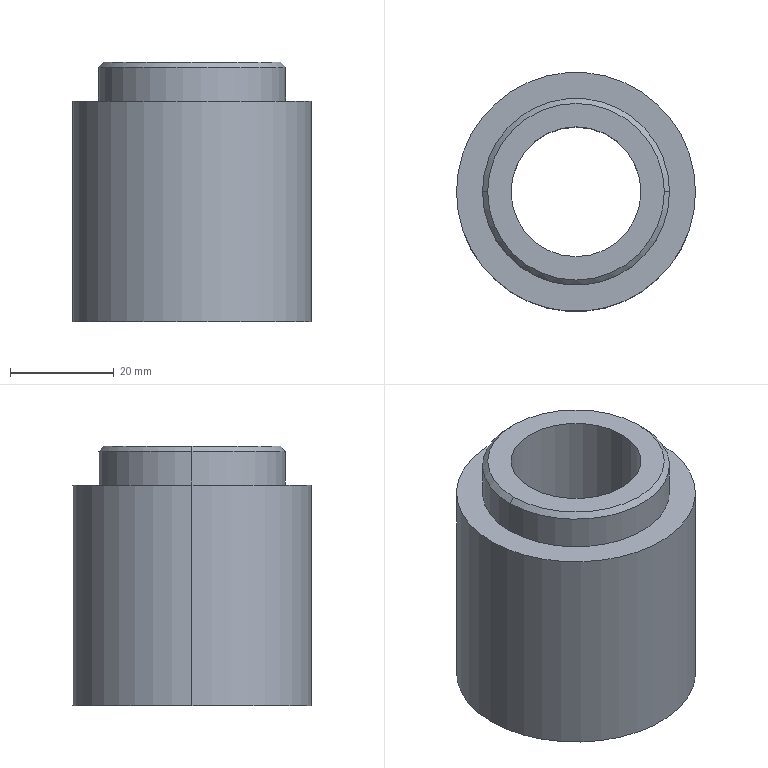Part | SolidWorks | features ICE 2, Chamfer 1, Extrusion 1 | 1 solid | 11 faces | box 46 x 46 x 50 mm | volume 53666 mm3 | cylinder 6 | plane 3 | cone 2 | commonest cylinder face diameters 25 x2 36 x2 46 x2
STEP:
#1=CARTESIAN_POINT('',(17.,0.,50.));
#2=VERTEX_POINT('',#1);
#3=CARTESIAN_POINT('',(-17.,0.,50.));
#4=VERTEX_POINT('',#3);
#5=CARTESIAN_POINT('',(0.,0.,50.));
#6=DIRECTION('',(0.,0.,1.));
#7=DIRECTION('',(1.,0.,0.));
#8=AXIS2_PLACEMENT_3D('',#5,#6,#7);
#9=CIRCLE('',#8,17.);
#10=EDGE_CURVE('',#2,#4,#9,.T.);
#11=ORIENTED_EDGE('',*,*,#10,.F.);
#12=CARTESIAN_POINT('',(18.,0.,49.));
#13=VERTEX_POINT('',#12);
#14=CARTESIAN_POINT('',(17.,0.,50.));
#15=DIRECTION('',(0.7071,0.,-0.7071));
#16=VECTOR('',#15,1000.);
#17=LINE('',#14,#16);
#18=EDGE_CURVE('',#2,#13,#17,.T.);
#19=ORIENTED_EDGE('',*,*,#18,.T.);
#20=CARTESIAN_POINT('',(-18.,0.,49.));
#21=VERTEX_POINT('',#20);
#22=CARTESIAN_POINT('',(0.,0.,49.));
#23=DIRECTION('',(0.,0.,-1.));
#24=DIRECTION('',(1.,0.,0.));
#25=AXIS2_PLACEMENT_3D('',#22,#23,#24);
#26=CIRCLE('',#25,18.);
#27=EDGE_CURVE('',#21,#13,#26,.T.);
#28=ORIENTED_EDGE('',*,*,#27,.F.);
#29=CARTESIAN_POINT('',(-17.,0.,50.));
#30=DIRECTION('',(-0.7071,0.,-0.7071));
#31=VECTOR('',#30,1000.);
#32=LINE('',#29,#31);
#33=EDGE_CURVE('',#4,#21,#32,.T.);
#34=ORIENTED_EDGE('',*,*,#33,.F.);
#35=EDGE_LOOP('',(#11,#19,#28,#34));
#36=FACE_OUTER_BOUND('',#35,.T.);
#37=CARTESIAN_POINT('',(0.,0.,50.));
#38=DIRECTION('',(0.,0.,-1.));
#39=DIRECTION('',(-1.,0.,0.));
#40=AXIS2_PLACEMENT_3D('',#37,#38,#39);
#41=CONICAL_SURFACE('',#40,17.,0.7854);
#42=ADVANCED_FACE('',(#36),#41,.T.);
#43=CARTESIAN_POINT('',(-12.5,0.,0.));
#44=VERTEX_POINT('',#43);
#45=CARTESIAN_POINT('',(12.5,0.,0.));
#46=VERTEX_POINT('',#45);
#47=CARTESIAN_POINT('',(0.,0.,0.));
#48=DIRECTION('',(0.,0.,1.));
#49=DIRECTION('',(1.,0.,0.));
#50=AXIS2_PLACEMENT_3D('',#47,#48,#49);
#51=CIRCLE('',#50,12.5);
#52=EDGE_CURVE('',#44,#46,#51,.T.);
#53=ORIENTED_EDGE('',*,*,#52,.F.);
#54=CARTESIAN_POINT('',(-12.5,0.,50.));
#55=VERTEX_POINT('',#54);
#56=CARTESIAN_POINT('',(-12.5,0.,0.));
#57=DIRECTION('',(0.,0.,1.));
#58=VECTOR('',#57,1000.);
#59=LINE('',#56,#58);
#60=EDGE_CURVE('',#44,#55,#59,.T.);
#61=ORIENTED_EDGE('',*,*,#60,.T.);
#62=CARTESIAN_POINT('',(12.5,0.,50.));
#63=VERTEX_POINT('',#62);
#64=CARTESIAN_POINT('',(0.,0.,50.));
#65=DIRECTION('',(0.,0.,1.));
#66=DIRECTION('',(1.,0.,0.));
#67=AXIS2_PLACEMENT_3D('',#64,#65,#66);
#68=CIRCLE('',#67,12.5);
#69=EDGE_CURVE('',#55,#63,#68,.T.);
#70=ORIENTED_EDGE('',*,*,#69,.T.);
#71=CARTESIAN_POINT('',(12.5,0.,0.));
#72=DIRECTION('',(0.,0.,1.));
#73=VECTOR('',#72,1000.);
#74=LINE('',#71,#73);
#75=EDGE_CURVE('',#46,#63,#74,.T.);
#76=ORIENTED_EDGE('',*,*,#75,.F.);
#77=EDGE_LOOP('',(#53,#61,#70,#76));
#78=FACE_OUTER_BOUND('',#77,.T.);
#79=CARTESIAN_POINT('',(0.,0.,0.));
#80=DIRECTION('',(0.,0.,1.));
#81=DIRECTION('',(1.,0.,0.));
#82=AXIS2_PLACEMENT_3D('',#79,#80,#81);
#83=CYLINDRICAL_SURFACE('',#82,12.5);
#84=ADVANCED_FACE('',(#78),#83,.F.);
#85=CARTESIAN_POINT('',(18.,0.,42.5));
#86=VERTEX_POINT('',#85);
#87=CARTESIAN_POINT('',(-18.,0.,42.5));
#88=VERTEX_POINT('',#87);
#89=CARTESIAN_POINT('',(0.,0.,42.5));
#90=DIRECTION('',(0.,0.,1.));
#91=DIRECTION('',(1.,0.,0.));
#92=AXIS2_PLACEMENT_3D('',#89,#90,#91);
#93=CIRCLE('',#92,18.);
#94=EDGE_CURVE('',#86,#88,#93,.T.);
#95=ORIENTED_EDGE('',*,*,#94,.T.);
#96=CARTESIAN_POINT('',(-18.,0.,42.5));
#97=DIRECTION('',(0.,0.,1.));
#98=VECTOR('',#97,1000.);
#99=LINE('',#96,#98);
#100=EDGE_CURVE('',#88,#21,#99,.T.);
#101=ORIENTED_EDGE('',*,*,#100,.T.);
#102=ORIENTED_EDGE('',*,*,#27,.T.);
#103=CARTESIAN_POINT('',(18.,0.,42.5));
#104=DIRECTION('',(0.,0.,1.));
#105=VECTOR('',#104,1000.);
#106=LINE('',#103,#105);
#107=EDGE_CURVE('',#86,#13,#106,.T.);
#108=ORIENTED_EDGE('',*,*,#107,.F.);
#109=EDGE_LOOP('',(#95,#101,#102,#108));
#110=FACE_OUTER_BOUND('',#109,.T.);
#111=CARTESIAN_POINT('',(0.,0.,42.5));
#112=DIRECTION('',(0.,0.,1.));
#113=DIRECTION('',(1.,0.,0.));
#114=AXIS2_PLACEMENT_3D('',#111,#112,#113);
#115=CYLINDRICAL_SURFACE('',#114,18.);
#116=ADVANCED_FACE('',(#110),#115,.T.);
#117=CARTESIAN_POINT('',(23.,0.,42.5));
#118=VERTEX_POINT('',#117);
#119=CARTESIAN_POINT('',(-23.,0.,42.5));
#120=VERTEX_POINT('',#119);
#121=CARTESIAN_POINT('',(0.,0.,42.5));
#122=DIRECTION('',(0.,0.,1.));
#123=DIRECTION('',(1.,0.,0.));
#124=AXIS2_PLACEMENT_3D('',#121,#122,#123);
#125=CIRCLE('',#124,23.);
#126=EDGE_CURVE('',#118,#120,#125,.T.);
#127=ORIENTED_EDGE('',*,*,#126,.F.);
#128=CARTESIAN_POINT('',(23.,0.,0.));
#129=VERTEX_POINT('',#128);
#130=CARTESIAN_POINT('',(23.,0.,50.));
#131=DIRECTION('',(0.,0.,-1.));
#132=VECTOR('',#131,1000.);
#133=LINE('',#130,#132);
#134=EDGE_CURVE('',#118,#129,#133,.T.);
#135=ORIENTED_EDGE('',*,*,#134,.T.);
#136=CARTESIAN_POINT('',(-23.,0.,0.));
#137=VERTEX_POINT('',#136);
#138=CARTESIAN_POINT('',(0.,0.,0.));
#139=DIRECTION('',(0.,0.,1.));
#140=DIRECTION('',(1.,0.,0.));
#141=AXIS2_PLACEMENT_3D('',#138,#139,#140);
#142=CIRCLE('',#141,23.);
#143=EDGE_CURVE('',#129,#137,#142,.T.);
#144=ORIENTED_EDGE('',*,*,#143,.T.);
#145=CARTESIAN_POINT('',(-23.,0.,50.));
#146=DIRECTION('',(0.,0.,-1.));
#147=VECTOR('',#146,1000.);
#148=LINE('',#145,#147);
#149=EDGE_CURVE('',#120,#137,#148,.T.);
#150=ORIENTED_EDGE('',*,*,#149,.F.);
#151=EDGE_LOOP('',(#127,#135,#144,#150));
#152=FACE_OUTER_BOUND('',#151,.T.);
#153=CARTESIAN_POINT('',(0.,0.,50.));
#154=DIRECTION('',(0.,0.,-1.));
#155=DIRECTION('',(-1.,0.,0.));
#156=AXIS2_PLACEMENT_3D('',#153,#154,#155);
#157=CYLINDRICAL_SURFACE('',#156,23.);
#158=ADVANCED_FACE('',(#152),#157,.T.);
#159=ORIENTED_EDGE('',*,*,#134,.F.);
#160=CARTESIAN_POINT('',(0.,0.,42.5));
#161=DIRECTION('',(0.,0.,1.));
#162=DIRECTION('',(1.,0.,0.));
#163=AXIS2_PLACEMENT_3D('',#160,#161,#162);
#164=CIRCLE('',#163,23.);
#165=EDGE_CURVE('',#120,#118,#164,.T.);
#166=ORIENTED_EDGE('',*,*,#165,.F.);
#167=ORIENTED_EDGE('',*,*,#149,.T.);
#168=CARTESIAN_POINT('',(0.,0.,0.));
#169=DIRECTION('',(0.,0.,1.));
#170=DIRECTION('',(1.,0.,0.));
#171=AXIS2_PLACEMENT_3D('',#168,#169,#170);
#172=CIRCLE('',#171,23.);
#173=EDGE_CURVE('',#137,#129,#172,.T.);
#174=ORIENTED_EDGE('',*,*,#173,.T.);
#175=EDGE_LOOP('',(#159,#166,#167,#174));
#176=FACE_OUTER_BOUND('',#175,.T.);
#177=CARTESIAN_POINT('',(0.,0.,50.));
#178=DIRECTION('',(0.,0.,-1.));
#179=DIRECTION('',(-1.,0.,0.));
#180=AXIS2_PLACEMENT_3D('',#177,#178,#179);
#181=CYLINDRICAL_SURFACE('',#180,23.);
#182=ADVANCED_FACE('',(#176),#181,.T.);
#183=CARTESIAN_POINT('',(0.,0.,0.));
#184=DIRECTION('',(0.,0.,1.));
#185=DIRECTION('',(1.,0.,0.));
#186=AXIS2_PLACEMENT_3D('',#183,#184,#185);
#187=CIRCLE('',#186,12.5);
#188=EDGE_CURVE('',#46,#44,#187,.T.);
#189=ORIENTED_EDGE('',*,*,#188,.T.);
#190=ORIENTED_EDGE('',*,*,#52,.T.);
#191=EDGE_LOOP('',(#189,#190));
#192=FACE_BOUND('',#191,.T.);
#193=ORIENTED_EDGE('',*,*,#173,.F.);
#194=ORIENTED_EDGE('',*,*,#143,.F.);
#195=EDGE_LOOP('',(#193,#194));
#196=FACE_OUTER_BOUND('',#195,.T.);
#197=CARTESIAN_POINT('',(0.,0.,0.));
#198=DIRECTION('',(0.,0.,1.));
#199=DIRECTION('',(1.,0.,0.));
#200=AXIS2_PLACEMENT_3D('',#197,#198,#199);
#201=PLANE('',#200);
#202=ADVANCED_FACE('',(#192,#196),#201,.F.);
#203=ORIENTED_EDGE('',*,*,#94,.F.);
#204=CARTESIAN_POINT('',(0.,0.,42.5));
#205=DIRECTION('',(0.,0.,1.));
#206=DIRECTION('',(1.,0.,0.));
#207=AXIS2_PLACEMENT_3D('',#204,#205,#206);
#208=CIRCLE('',#207,18.);
#209=EDGE_CURVE('',#88,#86,#208,.T.);
#210=ORIENTED_EDGE('',*,*,#209,.F.);
#211=EDGE_LOOP('',(#203,#210));
#212=FACE_BOUND('',#211,.T.);
#213=ORIENTED_EDGE('',*,*,#165,.T.);
#214=ORIENTED_EDGE('',*,*,#126,.T.);
#215=EDGE_LOOP('',(#213,#214));
#216=FACE_OUTER_BOUND('',#215,.T.);
#217=CARTESIAN_POINT('',(0.,0.,42.5));
#218=DIRECTION('',(0.,0.,1.));
#219=DIRECTION('',(1.,0.,0.));
#220=AXIS2_PLACEMENT_3D('',#217,#218,#219);
#221=PLANE('',#220);
#222=ADVANCED_FACE('',(#212,#216),#221,.T.);
#223=ORIENTED_EDGE('',*,*,#100,.F.);
#224=ORIENTED_EDGE('',*,*,#209,.T.);
#225=ORIENTED_EDGE('',*,*,#107,.T.);
#226=CARTESIAN_POINT('',(0.,0.,49.));
#227=DIRECTION('',(0.,0.,-1.));
#228=DIRECTION('',(1.,0.,0.));
#229=AXIS2_PLACEMENT_3D('',#226,#227,#228);
#230=CIRCLE('',#229,18.);
#231=EDGE_CURVE('',#13,#21,#230,.T.);
#232=ORIENTED_EDGE('',*,*,#231,.T.);
#233=EDGE_LOOP('',(#223,#224,#225,#232));
#234=FACE_OUTER_BOUND('',#233,.T.);
#235=CARTESIAN_POINT('',(0.,0.,42.5));
#236=DIRECTION('',(0.,0.,1.));
#237=DIRECTION('',(1.,0.,0.));
#238=AXIS2_PLACEMENT_3D('',#235,#236,#237);
#239=CYLINDRICAL_SURFACE('',#238,18.);
#240=ADVANCED_FACE('',(#234),#239,.T.);
#241=CARTESIAN_POINT('',(0.,0.,50.));
#242=DIRECTION('',(0.,0.,1.));
#243=DIRECTION('',(1.,0.,0.));
#244=AXIS2_PLACEMENT_3D('',#241,#242,#243);
#245=CIRCLE('',#244,17.);
#246=EDGE_CURVE('',#4,#2,#245,.T.);
#247=ORIENTED_EDGE('',*,*,#246,.T.);
#248=ORIENTED_EDGE('',*,*,#10,.T.);
#249=EDGE_LOOP('',(#247,#248));
#250=FACE_OUTER_BOUND('',#249,.T.);
#251=CARTESIAN_POINT('',(0.,0.,50.));
#252=DIRECTION('',(0.,0.,1.));
#253=DIRECTION('',(1.,0.,0.));
#254=AXIS2_PLACEMENT_3D('',#251,#252,#253);
#255=CIRCLE('',#254,12.5);
#256=EDGE_CURVE('',#63,#55,#255,.T.);
#257=ORIENTED_EDGE('',*,*,#256,.F.);
#258=ORIENTED_EDGE('',*,*,#69,.F.);
#259=EDGE_LOOP('',(#257,#258));
#260=FACE_BOUND('',#259,.T.);
#261=CARTESIAN_POINT('',(0.,0.,50.));
#262=DIRECTION('',(0.,0.,1.));
#263=DIRECTION('',(1.,0.,0.));
#264=AXIS2_PLACEMENT_3D('',#261,#262,#263);
#265=PLANE('',#264);
#266=ADVANCED_FACE('',(#250,#260),#265,.T.);
#267=ORIENTED_EDGE('',*,*,#60,.F.);
#268=ORIENTED_EDGE('',*,*,#188,.F.);
#269=ORIENTED_EDGE('',*,*,#75,.T.);
#270=ORIENTED_EDGE('',*,*,#256,.T.);
#271=EDGE_LOOP('',(#267,#268,#269,#270));
#272=FACE_OUTER_BOUND('',#271,.T.);
#273=CARTESIAN_POINT('',(0.,0.,0.));
#274=DIRECTION('',(0.,0.,1.));
#275=DIRECTION('',(1.,0.,0.));
#276=AXIS2_PLACEMENT_3D('',#273,#274,#275);
#277=CYLINDRICAL_SURFACE('',#276,12.5);
#278=ADVANCED_FACE('',(#272),#277,.F.);
#279=ORIENTED_EDGE('',*,*,#18,.F.);
#280=ORIENTED_EDGE('',*,*,#246,.F.);
#281=ORIENTED_EDGE('',*,*,#33,.T.);
#282=ORIENTED_EDGE('',*,*,#231,.F.);
#283=EDGE_LOOP('',(#279,#280,#281,#282));
#284=FACE_OUTER_BOUND('',#283,.T.);
#285=CARTESIAN_POINT('',(0.,0.,50.));
#286=DIRECTION('',(0.,0.,-1.));
#287=DIRECTION('',(-1.,0.,0.));
#288=AXIS2_PLACEMENT_3D('',#285,#286,#287);
#289=CONICAL_SURFACE('',#288,17.,0.7854);
#290=ADVANCED_FACE('',(#284),#289,.T.);
#291=CLOSED_SHELL('',(#42,#84,#116,#158,#182,#202,#222,#240,#266,#278,#290));
#292=MANIFOLD_SOLID_BREP('',#291);
#293=CARTESIAN_POINT('',(0.,0.,0.));
#294=DIRECTION('',(0.,0.,1.));
#295=DIRECTION('',(1.,0.,0.));
#296=AXIS2_PLACEMENT_3D('',#293,#294,#295);
#297=(LENGTH_UNIT()NAMED_UNIT(*)SI_UNIT(.MILLI.,.METRE.));
#298=UNCERTAINTY_MEASURE_WITH_UNIT(LENGTH_MEASURE(0.00001),#297,'','');
#299=(NAMED_UNIT(*)PLANE_ANGLE_UNIT()SI_UNIT($,.RADIAN.));
#300=(NAMED_UNIT(*)SI_UNIT($,.STERADIAN.)SOLID_ANGLE_UNIT());
#301=(GEOMETRIC_REPRESENTATION_CONTEXT(3)GLOBAL_UNCERTAINTY_ASSIGNED_CONTEXT((#298))GLOBAL_UNIT_ASSIGNED_CONTEXT((#297,#299,#300))REPRESENTATION_CONTEXT('',''));
#302=ADVANCED_BREP_SHAPE_REPRESENTATION('',(#292,#296),#301);